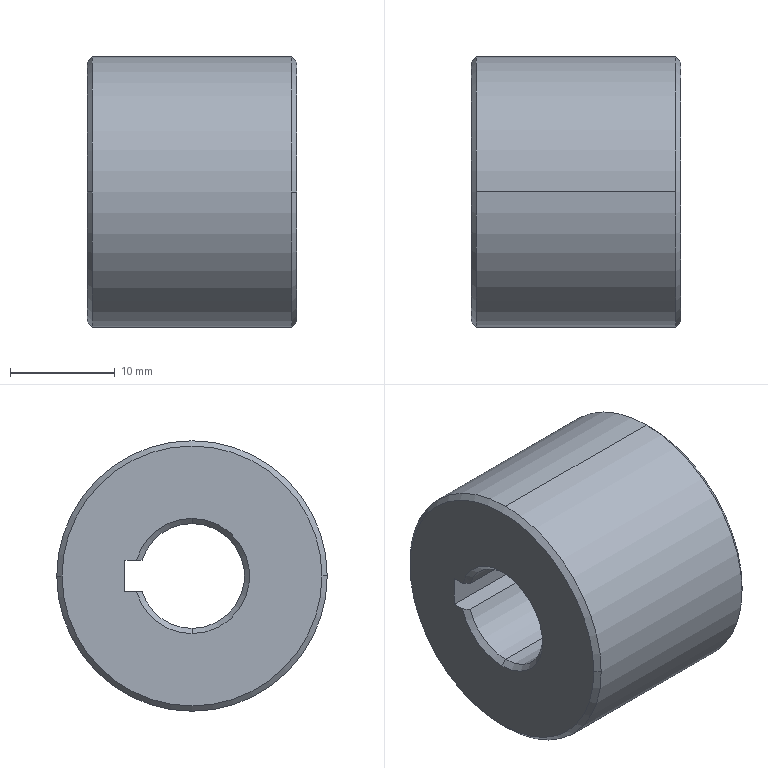Part | STEP file | 06-02 Support feed wheel | 1 solid | 20 faces | box 20 x 25.8 x 25.8 mm | volume 8769 mm3 | cone 10 | cylinder 5 | plane 5 | commonest cylinder face diameters 10 x3 25.8 x2